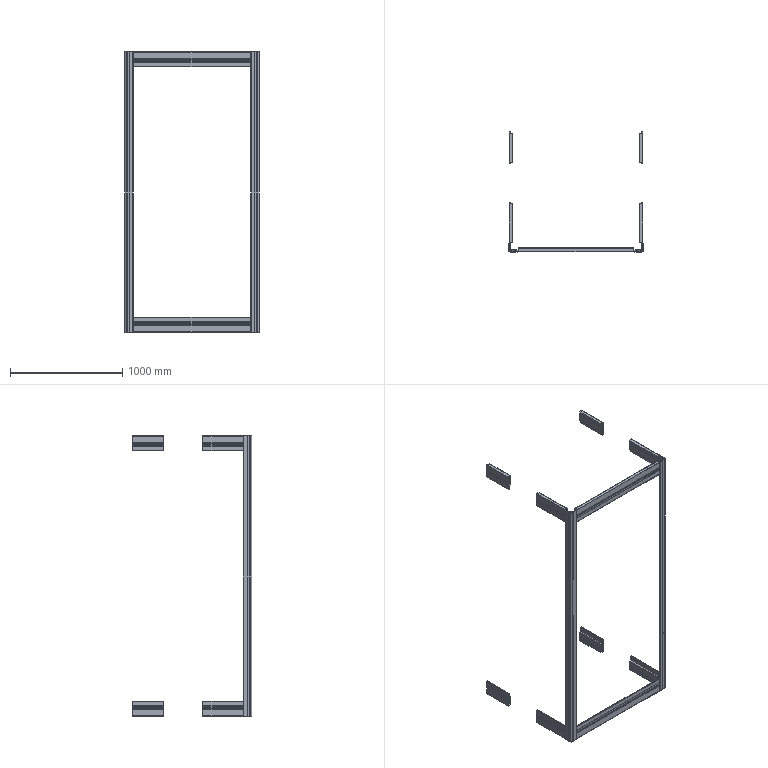Part | SolidWorks | features ICE 4, MirrorPattern 2, WeldMemberFeat 2, 3DProfileFeature 1, Cut 1, WeldmentFeature 1 | 12 solids | 803 faces | box 1199 x 1067 x 2502 mm | volume 8436439 mm3 | plane 688 | cylinder 115 | commonest cylinder face diameters 0.4 x70 10 x32 26 x6 2 x4 18 x3